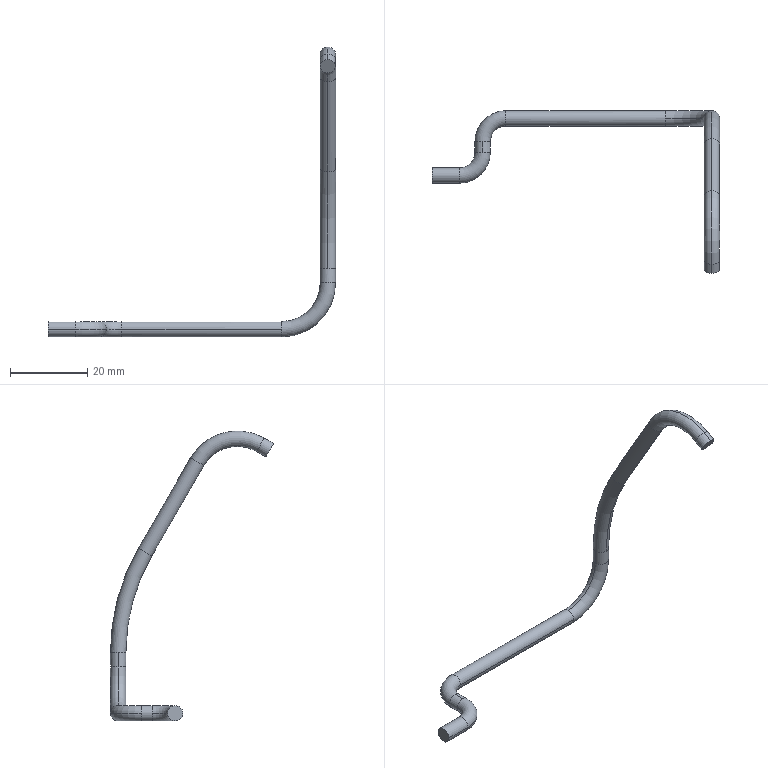Part | SolidWorks | features 3DProfileFeature 2, Sweep 1 | 1 solid | 24 faces | box 74.439 x 42.263 x 75.178 mm | volume 2118 mm3 | cylinder 12 | torus 10 | plane 2 | commonest cylinder face diameters 4 x12
STEP:
#1=CARTESIAN_POINT('',(-50.159,50.824,64.286));
#2=VERTEX_POINT('',#1);
#3=CARTESIAN_POINT('',(-50.154,54.288,66.285));
#4=VERTEX_POINT('',#3);
#5=CARTESIAN_POINT('',(-50.159,52.556,65.286));
#6=DIRECTION('',(0.,-0.4999,0.8661));
#7=DIRECTION('',(1.,0.,0.));
#8=AXIS2_PLACEMENT_3D('',#5,#6,#7);
#9=CIRCLE('',#8,2.);
#10=EDGE_CURVE('',#2,#4,#9,.T.);
#11=ORIENTED_EDGE('',*,*,#10,.T.);
#12=CARTESIAN_POINT('',(-50.191,35.164,71.413));
#13=VERTEX_POINT('',#12);
#14=CARTESIAN_POINT('',(-50.191,42.163,59.287));
#15=DIRECTION('',(1.,-0.00231,-0.001333));
#16=DIRECTION('',(0.00231,1.,0.));
#17=AXIS2_PLACEMENT_3D('',#14,#15,#16);
#18=CIRCLE('',#17,14.);
#19=EDGE_CURVE('',#4,#13,#18,.T.);
#20=ORIENTED_EDGE('',*,*,#19,.T.);
#21=CARTESIAN_POINT('',(-50.191,37.164,67.948));
#22=VERTEX_POINT('',#21);
#23=CARTESIAN_POINT('',(-50.191,36.164,69.681));
#24=DIRECTION('',(-0.002667,-0.8661,-0.4999));
#25=DIRECTION('',(1.,-0.003643,0.0009767));
#26=AXIS2_PLACEMENT_3D('',#23,#24,#25);
#27=CIRCLE('',#26,2.);
#28=EDGE_CURVE('',#22,#13,#27,.T.);
#29=ORIENTED_EDGE('',*,*,#28,.F.);
#30=CARTESIAN_POINT('',(-50.164,50.824,64.286));
#31=VERTEX_POINT('',#30);
#32=CARTESIAN_POINT('',(-50.191,42.163,59.287));
#33=DIRECTION('',(1.,-0.00231,-0.001333));
#34=DIRECTION('',(0.00231,1.,0.));
#35=AXIS2_PLACEMENT_3D('',#32,#33,#34);
#36=CIRCLE('',#35,10.);
#37=EDGE_CURVE('',#31,#22,#36,.T.);
#38=ORIENTED_EDGE('',*,*,#37,.F.);
#39=CARTESIAN_POINT('',(-50.159,52.556,65.286));
#40=DIRECTION('',(0.,-0.4999,0.8661));
#41=DIRECTION('',(1.,0.,0.));
#42=AXIS2_PLACEMENT_3D('',#39,#40,#41);
#43=CIRCLE('',#42,2.);
#44=EDGE_CURVE('',#31,#2,#43,.T.);
#45=ORIENTED_EDGE('',*,*,#44,.T.);
#46=EDGE_LOOP('',(#11,#20,#29,#38,#45));
#47=FACE_OUTER_BOUND('',#46,.T.);
#48=CARTESIAN_POINT('',(-50.191,42.163,59.287));
#49=DIRECTION('',(1.,-0.00231,-0.001333));
#50=DIRECTION('',(0.00231,1.,0.));
#51=AXIS2_PLACEMENT_3D('',#48,#49,#50);
#52=TOROIDAL_SURFACE('',#51,12.,2.);
#53=ADVANCED_FACE('',(#47),#52,.T.);
#54=CARTESIAN_POINT('',(-48.159,73.044,15.858));
#55=VERTEX_POINT('',#54);
#56=CARTESIAN_POINT('',(-50.159,75.044,15.858));
#57=VERTEX_POINT('',#56);
#58=CARTESIAN_POINT('',(-50.159,73.044,15.858));
#59=DIRECTION('',(0.,0.,1.));
#60=DIRECTION('',(1.,0.,0.));
#61=AXIS2_PLACEMENT_3D('',#58,#59,#60);
#62=CIRCLE('',#61,2.);
#63=EDGE_CURVE('',#55,#57,#62,.T.);
#64=ORIENTED_EDGE('',*,*,#63,.T.);
#65=CARTESIAN_POINT('',(-50.159,67.813,42.851));
#66=VERTEX_POINT('',#65);
#67=CARTESIAN_POINT('',(-50.159,21.044,15.858));
#68=DIRECTION('',(1.,0.,0.));
#69=DIRECTION('',(0.,0.,-1.));
#70=AXIS2_PLACEMENT_3D('',#67,#68,#69);
#71=CIRCLE('',#70,54.);
#72=EDGE_CURVE('',#57,#66,#71,.T.);
#73=ORIENTED_EDGE('',*,*,#72,.T.);
#74=CARTESIAN_POINT('',(-50.159,64.349,40.852));
#75=VERTEX_POINT('',#74);
#76=CARTESIAN_POINT('',(-50.159,66.081,41.851));
#77=DIRECTION('',(0.,-0.4999,0.8661));
#78=DIRECTION('',(1.,0.,0.));
#79=AXIS2_PLACEMENT_3D('',#76,#77,#78);
#80=CIRCLE('',#79,2.);
#81=EDGE_CURVE('',#75,#66,#80,.T.);
#82=ORIENTED_EDGE('',*,*,#81,.F.);
#83=CARTESIAN_POINT('',(-50.159,71.044,15.858));
#84=VERTEX_POINT('',#83);
#85=CARTESIAN_POINT('',(-50.159,21.044,15.858));
#86=DIRECTION('',(1.,0.,0.));
#87=DIRECTION('',(0.,0.,-1.));
#88=AXIS2_PLACEMENT_3D('',#85,#86,#87);
#89=CIRCLE('',#88,50.);
#90=EDGE_CURVE('',#84,#75,#89,.T.);
#91=ORIENTED_EDGE('',*,*,#90,.F.);
#92=CARTESIAN_POINT('',(-50.159,73.044,15.858));
#93=DIRECTION('',(0.,0.,1.));
#94=DIRECTION('',(1.,0.,0.));
#95=AXIS2_PLACEMENT_3D('',#92,#93,#94);
#96=CIRCLE('',#95,2.);
#97=EDGE_CURVE('',#84,#55,#96,.T.);
#98=ORIENTED_EDGE('',*,*,#97,.T.);
#99=EDGE_LOOP('',(#64,#73,#82,#91,#98));
#100=FACE_OUTER_BOUND('',#99,.T.);
#101=CARTESIAN_POINT('',(-50.159,21.044,15.858));
#102=DIRECTION('',(1.,0.,0.));
#103=DIRECTION('',(0.,0.,-1.));
#104=AXIS2_PLACEMENT_3D('',#101,#102,#103);
#105=TOROIDAL_SURFACE('',#104,52.,2.);
#106=ADVANCED_FACE('',(#100),#105,.T.);
#107=CARTESIAN_POINT('',(-62.159,71.044,0.1096));
#108=VERTEX_POINT('',#107);
#109=CARTESIAN_POINT('',(-62.159,73.044,-1.89));
#110=VERTEX_POINT('',#109);
#111=CARTESIAN_POINT('',(-62.159,73.044,0.1096));
#112=DIRECTION('',(1.,0.,0.));
#113=DIRECTION('',(0.,0.,-1.));
#114=AXIS2_PLACEMENT_3D('',#111,#112,#113);
#115=CIRCLE('',#114,2.);
#116=EDGE_CURVE('',#108,#110,#115,.T.);
#117=ORIENTED_EDGE('',*,*,#116,.T.);
#118=CARTESIAN_POINT('',(-48.159,73.044,12.11));
#119=VERTEX_POINT('',#118);
#120=CARTESIAN_POINT('',(-62.159,73.044,12.11));
#121=DIRECTION('',(0.,-1.,0.));
#122=DIRECTION('',(0.,0.,-1.));
#123=AXIS2_PLACEMENT_3D('',#120,#121,#122);
#124=CIRCLE('',#123,14.);
#125=EDGE_CURVE('',#110,#119,#124,.T.);
#126=ORIENTED_EDGE('',*,*,#125,.T.);
#127=CARTESIAN_POINT('',(-52.159,73.044,12.11));
#128=VERTEX_POINT('',#127);
#129=CARTESIAN_POINT('',(-50.159,73.044,12.11));
#130=DIRECTION('',(0.,0.,1.));
#131=DIRECTION('',(1.,0.,0.));
#132=AXIS2_PLACEMENT_3D('',#129,#130,#131);
#133=CIRCLE('',#132,2.);
#134=EDGE_CURVE('',#128,#119,#133,.T.);
#135=ORIENTED_EDGE('',*,*,#134,.F.);
#136=CARTESIAN_POINT('',(-62.159,73.044,2.11));
#137=VERTEX_POINT('',#136);
#138=CARTESIAN_POINT('',(-62.159,73.044,12.11));
#139=DIRECTION('',(0.,-1.,0.));
#140=DIRECTION('',(0.,0.,-1.));
#141=AXIS2_PLACEMENT_3D('',#138,#139,#140);
#142=CIRCLE('',#141,10.);
#143=EDGE_CURVE('',#137,#128,#142,.T.);
#144=ORIENTED_EDGE('',*,*,#143,.F.);
#145=CARTESIAN_POINT('',(-62.159,73.044,0.1096));
#146=DIRECTION('',(1.,0.,0.));
#147=DIRECTION('',(0.,0.,-1.));
#148=AXIS2_PLACEMENT_3D('',#145,#146,#147);
#149=CIRCLE('',#148,2.);
#150=EDGE_CURVE('',#137,#108,#149,.T.);
#151=ORIENTED_EDGE('',*,*,#150,.T.);
#152=EDGE_LOOP('',(#117,#126,#135,#144,#151));
#153=FACE_OUTER_BOUND('',#152,.T.);
#154=CARTESIAN_POINT('',(-62.159,73.044,12.11));
#155=DIRECTION('',(0.,-1.,0.));
#156=DIRECTION('',(0.,0.,-1.));
#157=AXIS2_PLACEMENT_3D('',#154,#155,#156);
#158=TOROIDAL_SURFACE('',#157,12.,2.);
#159=ADVANCED_FACE('',(#153),#158,.T.);
#160=CARTESIAN_POINT('',(-109.578,67.044,-1.89));
#161=VERTEX_POINT('',#160);
#162=CARTESIAN_POINT('',(-111.578,67.044,0.1096));
#163=VERTEX_POINT('',#162);
#164=CARTESIAN_POINT('',(-109.578,67.044,0.1096));
#165=DIRECTION('',(0.,1.,0.));
#166=DIRECTION('',(0.,0.,-1.));
#167=AXIS2_PLACEMENT_3D('',#164,#165,#166);
#168=CIRCLE('',#167,2.);
#169=EDGE_CURVE('',#161,#163,#168,.T.);
#170=ORIENTED_EDGE('',*,*,#169,.T.);
#171=CARTESIAN_POINT('',(-103.578,75.044,0.1096));
#172=VERTEX_POINT('',#171);
#173=CARTESIAN_POINT('',(-103.578,67.044,0.1096));
#174=DIRECTION('',(0.,0.,-1.));
#175=DIRECTION('',(-1.,0.,0.));
#176=AXIS2_PLACEMENT_3D('',#173,#174,#175);
#177=CIRCLE('',#176,8.);
#178=EDGE_CURVE('',#163,#172,#177,.T.);
#179=ORIENTED_EDGE('',*,*,#178,.T.);
#180=CARTESIAN_POINT('',(-103.578,71.044,0.1096));
#181=VERTEX_POINT('',#180);
#182=CARTESIAN_POINT('',(-103.578,73.044,0.1096));
#183=DIRECTION('',(1.,0.,0.));
#184=DIRECTION('',(0.,0.,-1.));
#185=AXIS2_PLACEMENT_3D('',#182,#183,#184);
#186=CIRCLE('',#185,2.);
#187=EDGE_CURVE('',#181,#172,#186,.T.);
#188=ORIENTED_EDGE('',*,*,#187,.F.);
#189=CARTESIAN_POINT('',(-107.578,67.044,0.1096));
#190=VERTEX_POINT('',#189);
#191=CARTESIAN_POINT('',(-103.578,67.044,0.1096));
#192=DIRECTION('',(0.,0.,-1.));
#193=DIRECTION('',(-1.,0.,0.));
#194=AXIS2_PLACEMENT_3D('',#191,#192,#193);
#195=CIRCLE('',#194,4.);
#196=EDGE_CURVE('',#190,#181,#195,.T.);
#197=ORIENTED_EDGE('',*,*,#196,.F.);
#198=CARTESIAN_POINT('',(-109.578,67.044,0.1096));
#199=DIRECTION('',(0.,1.,0.));
#200=DIRECTION('',(0.,0.,-1.));
#201=AXIS2_PLACEMENT_3D('',#198,#199,#200);
#202=CIRCLE('',#201,2.);
#203=EDGE_CURVE('',#190,#161,#202,.T.);
#204=ORIENTED_EDGE('',*,*,#203,.T.);
#205=EDGE_LOOP('',(#170,#179,#188,#197,#204));
#206=FACE_OUTER_BOUND('',#205,.T.);
#207=CARTESIAN_POINT('',(-103.578,67.044,0.1096));
#208=DIRECTION('',(0.,0.,-1.));
#209=DIRECTION('',(-1.,0.,0.));
#210=AXIS2_PLACEMENT_3D('',#207,#208,#209);
#211=TOROIDAL_SURFACE('',#210,6.,2.);
#212=ADVANCED_FACE('',(#206),#211,.T.);
#213=CARTESIAN_POINT('',(-115.578,60.264,0.1096));
#214=VERTEX_POINT('',#213);
#215=CARTESIAN_POINT('',(-115.578,56.264,0.1096));
#216=VERTEX_POINT('',#215);
#217=CARTESIAN_POINT('',(-115.578,58.264,0.1096));
#218=DIRECTION('',(1.,0.,0.));
#219=DIRECTION('',(0.,0.,-1.));
#220=AXIS2_PLACEMENT_3D('',#217,#218,#219);
#221=CIRCLE('',#220,2.);
#222=EDGE_CURVE('',#214,#216,#221,.T.);
#223=ORIENTED_EDGE('',*,*,#222,.T.);
#224=CARTESIAN_POINT('',(-107.578,64.264,0.1096));
#225=VERTEX_POINT('',#224);
#226=CARTESIAN_POINT('',(-115.578,64.264,0.1096));
#227=DIRECTION('',(0.,0.,1.));
#228=DIRECTION('',(1.,0.,0.));
#229=AXIS2_PLACEMENT_3D('',#226,#227,#228);
#230=CIRCLE('',#229,8.);
#231=EDGE_CURVE('',#216,#225,#230,.T.);
#232=ORIENTED_EDGE('',*,*,#231,.T.);
#233=CARTESIAN_POINT('',(-109.578,64.264,2.11));
#234=VERTEX_POINT('',#233);
#235=CARTESIAN_POINT('',(-109.578,64.264,0.1096));
#236=DIRECTION('',(0.,1.,0.));
#237=DIRECTION('',(0.,0.,-1.));
#238=AXIS2_PLACEMENT_3D('',#235,#236,#237);
#239=CIRCLE('',#238,2.);
#240=EDGE_CURVE('',#234,#225,#239,.T.);
#241=ORIENTED_EDGE('',*,*,#240,.F.);
#242=CARTESIAN_POINT('',(-111.578,64.264,0.1096));
#243=VERTEX_POINT('',#242);
#244=CARTESIAN_POINT('',(-109.578,64.264,0.1096));
#245=DIRECTION('',(0.,1.,0.));
#246=DIRECTION('',(0.,0.,-1.));
#247=AXIS2_PLACEMENT_3D('',#244,#245,#246);
#248=CIRCLE('',#247,2.);
#249=EDGE_CURVE('',#243,#234,#248,.T.);
#250=ORIENTED_EDGE('',*,*,#249,.F.);
#251=CARTESIAN_POINT('',(-115.578,64.264,0.1096));
#252=DIRECTION('',(0.,0.,1.));
#253=DIRECTION('',(1.,0.,0.));
#254=AXIS2_PLACEMENT_3D('',#251,#252,#253);
#255=CIRCLE('',#254,4.);
#256=EDGE_CURVE('',#214,#243,#255,.T.);
#257=ORIENTED_EDGE('',*,*,#256,.F.);
#258=EDGE_LOOP('',(#223,#232,#241,#250,#257));
#259=FACE_OUTER_BOUND('',#258,.T.);
#260=CARTESIAN_POINT('',(-115.578,64.264,0.1096));
#261=DIRECTION('',(0.,0.,1.));
#262=DIRECTION('',(1.,0.,0.));
#263=AXIS2_PLACEMENT_3D('',#260,#261,#262);
#264=TOROIDAL_SURFACE('',#263,6.,2.);
#265=ADVANCED_FACE('',(#259),#264,.T.);
#266=ORIENTED_EDGE('',*,*,#28,.T.);
#267=CARTESIAN_POINT('',(-50.198,32.78,70.037));
#268=VERTEX_POINT('',#267);
#269=CARTESIAN_POINT('',(-50.191,35.164,71.413));
#270=DIRECTION('',(-0.002667,-0.8661,-0.4999));
#271=VECTOR('',#270,1000.);
#272=LINE('',#269,#271);
#273=EDGE_CURVE('',#13,#268,#272,.T.);
#274=ORIENTED_EDGE('',*,*,#273,.T.);
#275=CARTESIAN_POINT('',(-50.198,34.78,66.572));
#276=VERTEX_POINT('',#275);
#277=CARTESIAN_POINT('',(-50.198,33.78,68.304));
#278=DIRECTION('',(-0.002667,-0.8661,-0.4999));
#279=DIRECTION('',(1.,-0.003643,0.0009767));
#280=AXIS2_PLACEMENT_3D('',#277,#278,#279);
#281=CIRCLE('',#280,2.);
#282=EDGE_CURVE('',#276,#268,#281,.T.);
#283=ORIENTED_EDGE('',*,*,#282,.F.);
#284=CARTESIAN_POINT('',(-50.191,37.164,67.948));
#285=DIRECTION('',(-0.002667,-0.8661,-0.4999));
#286=VECTOR('',#285,1000.);
#287=LINE('',#284,#286);
#288=EDGE_CURVE('',#22,#276,#287,.T.);
#289=ORIENTED_EDGE('',*,*,#288,.F.);
#290=EDGE_LOOP('',(#266,#274,#283,#289));
#291=FACE_OUTER_BOUND('',#290,.T.);
#292=CARTESIAN_POINT('',(-50.191,36.164,69.681));
#293=DIRECTION('',(-0.002667,-0.8661,-0.4999));
#294=DIRECTION('',(0.,0.4999,-0.8661));
#295=AXIS2_PLACEMENT_3D('',#292,#293,#294);
#296=CYLINDRICAL_SURFACE('',#295,2.);
#297=ADVANCED_FACE('',(#291),#296,.T.);
#298=ORIENTED_EDGE('',*,*,#81,.T.);
#299=CARTESIAN_POINT('',(-50.159,54.288,66.285));
#300=VERTEX_POINT('',#299);
#301=CARTESIAN_POINT('',(-50.159,67.813,42.851));
#302=DIRECTION('',(0.,-0.4999,0.8661));
#303=VECTOR('',#302,1000.);
#304=LINE('',#301,#303);
#305=EDGE_CURVE('',#66,#300,#304,.T.);
#306=ORIENTED_EDGE('',*,*,#305,.T.);
#307=CARTESIAN_POINT('',(-50.159,52.556,65.286));
#308=DIRECTION('',(0.,-0.4999,0.8661));
#309=DIRECTION('',(1.,0.,0.));
#310=AXIS2_PLACEMENT_3D('',#307,#308,#309);
#311=CIRCLE('',#310,2.);
#312=EDGE_CURVE('',#4,#300,#311,.T.);
#313=ORIENTED_EDGE('',*,*,#312,.F.);
#314=ORIENTED_EDGE('',*,*,#10,.F.);
#315=CARTESIAN_POINT('',(-50.159,64.349,40.852));
#316=DIRECTION('',(0.,-0.4999,0.8661));
#317=VECTOR('',#316,1000.);
#318=LINE('',#315,#317);
#319=EDGE_CURVE('',#75,#2,#318,.T.);
#320=ORIENTED_EDGE('',*,*,#319,.F.);
#321=EDGE_LOOP('',(#298,#306,#313,#314,#320));
#322=FACE_OUTER_BOUND('',#321,.T.);
#323=CARTESIAN_POINT('',(-50.159,66.081,41.851));
#324=DIRECTION('',(0.,-0.4999,0.8661));
#325=DIRECTION('',(0.,-0.8661,-0.4999));
#326=AXIS2_PLACEMENT_3D('',#323,#324,#325);
#327=CYLINDRICAL_SURFACE('',#326,2.);
#328=ADVANCED_FACE('',(#322),#327,.T.);
#329=CARTESIAN_POINT('',(-50.159,73.044,12.11));
#330=DIRECTION('',(0.,0.,1.));
#331=DIRECTION('',(1.,0.,0.));
#332=AXIS2_PLACEMENT_3D('',#329,#330,#331);
#333=CIRCLE('',#332,2.);
#334=EDGE_CURVE('',#119,#128,#333,.T.);
#335=ORIENTED_EDGE('',*,*,#334,.T.);
#336=CARTESIAN_POINT('',(-52.159,73.044,15.858));
#337=VERTEX_POINT('',#336);
#338=CARTESIAN_POINT('',(-52.159,73.044,12.11));
#339=DIRECTION('',(0.,0.,1.));
#340=VECTOR('',#339,1000.);
#341=LINE('',#338,#340);
#342=EDGE_CURVE('',#128,#337,#341,.T.);
#343=ORIENTED_EDGE('',*,*,#342,.T.);
#344=CARTESIAN_POINT('',(-50.159,73.044,15.858));
#345=DIRECTION('',(0.,0.,1.));
#346=DIRECTION('',(1.,0.,0.));
#347=AXIS2_PLACEMENT_3D('',#344,#345,#346);
#348=CIRCLE('',#347,2.);
#349=EDGE_CURVE('',#57,#337,#348,.T.);
#350=ORIENTED_EDGE('',*,*,#349,.F.);
#351=ORIENTED_EDGE('',*,*,#63,.F.);
#352=CARTESIAN_POINT('',(-48.159,73.044,12.11));
#353=DIRECTION('',(0.,0.,1.));
#354=VECTOR('',#353,1000.);
#355=LINE('',#352,#354);
#356=EDGE_CURVE('',#119,#55,#355,.T.);
#357=ORIENTED_EDGE('',*,*,#356,.F.);
#358=EDGE_LOOP('',(#335,#343,#350,#351,#357));
#359=FACE_OUTER_BOUND('',#358,.T.);
#360=CARTESIAN_POINT('',(-50.159,73.044,12.11));
#361=DIRECTION('',(0.,0.,1.));
#362=DIRECTION('',(1.,0.,0.));
#363=AXIS2_PLACEMENT_3D('',#360,#361,#362);
#364=CYLINDRICAL_SURFACE('',#363,2.);
#365=ADVANCED_FACE('',(#359),#364,.T.);
#366=CARTESIAN_POINT('',(-103.578,73.044,0.1096));
#367=DIRECTION('',(1.,0.,0.));
#368=DIRECTION('',(0.,0.,-1.));
#369=AXIS2_PLACEMENT_3D('',#366,#367,#368);
#370=CIRCLE('',#369,2.);
#371=EDGE_CURVE('',#172,#181,#370,.T.);
#372=ORIENTED_EDGE('',*,*,#371,.T.);
#373=CARTESIAN_POINT('',(-103.578,71.044,0.1096));
#374=DIRECTION('',(1.,0.,0.));
#375=VECTOR('',#374,1000.);
#376=LINE('',#373,#375);
#377=EDGE_CURVE('',#181,#108,#376,.T.);
#378=ORIENTED_EDGE('',*,*,#377,.T.);
#379=ORIENTED_EDGE('',*,*,#150,.F.);
#380=CARTESIAN_POINT('',(-62.159,75.044,0.1096));
#381=VERTEX_POINT('',#380);
#382=CARTESIAN_POINT('',(-62.159,73.044,0.1096));
#383=DIRECTION('',(1.,0.,0.));
#384=DIRECTION('',(0.,0.,-1.));
#385=AXIS2_PLACEMENT_3D('',#382,#383,#384);
#386=CIRCLE('',#385,2.);
#387=EDGE_CURVE('',#381,#137,#386,.T.);
#388=ORIENTED_EDGE('',*,*,#387,.F.);
#389=CARTESIAN_POINT('',(-103.578,75.044,0.1096));
#390=DIRECTION('',(1.,0.,0.));
#391=VECTOR('',#390,1000.);
#392=LINE('',#389,#391);
#393=EDGE_CURVE('',#172,#381,#392,.T.);
#394=ORIENTED_EDGE('',*,*,#393,.F.);
#395=EDGE_LOOP('',(#372,#378,#379,#388,#394));
#396=FACE_OUTER_BOUND('',#395,.T.);
#397=CARTESIAN_POINT('',(-103.578,73.044,0.1096));
#398=DIRECTION('',(1.,0.,0.));
#399=DIRECTION('',(0.,1.,0.));
#400=AXIS2_PLACEMENT_3D('',#397,#398,#399);
#401=CYLINDRICAL_SURFACE('',#400,2.);
#402=ADVANCED_FACE('',(#396),#401,.T.);
#403=ORIENTED_EDGE('',*,*,#240,.T.);
#404=CARTESIAN_POINT('',(-109.578,64.264,-1.89));
#405=VERTEX_POINT('',#404);
#406=CARTESIAN_POINT('',(-109.578,64.264,0.1096));
#407=DIRECTION('',(0.,1.,0.));
#408=DIRECTION('',(0.,0.,-1.));
#409=AXIS2_PLACEMENT_3D('',#406,#407,#408);
#410=CIRCLE('',#409,2.);
#411=EDGE_CURVE('',#225,#405,#410,.T.);
#412=ORIENTED_EDGE('',*,*,#411,.T.);
#413=CARTESIAN_POINT('',(-109.578,64.264,-1.89));
#414=DIRECTION('',(0.,1.,0.));
#415=VECTOR('',#414,1000.);
#416=LINE('',#413,#415);
#417=EDGE_CURVE('',#405,#161,#416,.T.);
#418=ORIENTED_EDGE('',*,*,#417,.T.);
#419=ORIENTED_EDGE('',*,*,#203,.F.);
#420=CARTESIAN_POINT('',(-109.578,67.044,2.11));
#421=VERTEX_POINT('',#420);
#422=CARTESIAN_POINT('',(-109.578,67.044,0.1096));
#423=DIRECTION('',(0.,1.,0.));
#424=DIRECTION('',(0.,0.,-1.));
#425=AXIS2_PLACEMENT_3D('',#422,#423,#424);
#426=CIRCLE('',#425,2.);
#427=EDGE_CURVE('',#421,#190,#426,.T.);
#428=ORIENTED_EDGE('',*,*,#427,.F.);
#429=CARTESIAN_POINT('',(-109.578,64.264,2.11));
#430=DIRECTION('',(0.,1.,0.));
#431=VECTOR('',#430,1000.);
#432=LINE('',#429,#431);
#433=EDGE_CURVE('',#234,#421,#432,.T.);
#434=ORIENTED_EDGE('',*,*,#433,.F.);
#435=EDGE_LOOP('',(#403,#412,#418,#419,#428,#434));
#436=FACE_OUTER_BOUND('',#435,.T.);
#437=CARTESIAN_POINT('',(-109.578,64.264,0.1096));
#438=DIRECTION('',(0.,1.,0.));
#439=DIRECTION('',(0.,0.,1.));
#440=AXIS2_PLACEMENT_3D('',#437,#438,#439);
#441=CYLINDRICAL_SURFACE('',#440,2.);
#442=ADVANCED_FACE('',(#436),#441,.T.);
#443=CARTESIAN_POINT('',(-122.598,60.264,0.1096));
#444=VERTEX_POINT('',#443);
#445=CARTESIAN_POINT('',(-122.598,56.264,0.1096));
#446=VERTEX_POINT('',#445);
#447=CARTESIAN_POINT('',(-122.598,58.264,0.1096));
#448=DIRECTION('',(1.,0.,0.));
#449=DIRECTION('',(0.,0.,-1.));
#450=AXIS2_PLACEMENT_3D('',#447,#448,#449);
#451=CIRCLE('',#450,2.);
#452=EDGE_CURVE('',#444,#446,#451,.T.);
#453=ORIENTED_EDGE('',*,*,#452,.T.);
#454=CARTESIAN_POINT('',(-122.598,56.264,0.1096));
#455=DIRECTION('',(1.,0.,0.));
#456=VECTOR('',#455,1000.);
#457=LINE('',#454,#456);
#458=EDGE_CURVE('',#446,#216,#457,.T.);
#459=ORIENTED_EDGE('',*,*,#458,.T.);
#460=ORIENTED_EDGE('',*,*,#222,.F.);
#461=CARTESIAN_POINT('',(-122.598,60.264,0.1096));
#462=DIRECTION('',(1.,0.,0.));
#463=VECTOR('',#462,1000.);
#464=LINE('',#461,#463);
#465=EDGE_CURVE('',#444,#214,#464,.T.);
#466=ORIENTED_EDGE('',*,*,#465,.F.);
#467=EDGE_LOOP('',(#453,#459,#460,#466));
#468=FACE_OUTER_BOUND('',#467,.T.);
#469=CARTESIAN_POINT('',(-122.598,58.264,0.1096));
#470=DIRECTION('',(1.,0.,0.));
#471=DIRECTION('',(0.,1.,0.));
#472=AXIS2_PLACEMENT_3D('',#469,#470,#471);
#473=CYLINDRICAL_SURFACE('',#472,2.);
#474=ADVANCED_FACE('',(#468),#473,.T.);
#475=ORIENTED_EDGE('',*,*,#273,.F.);
#476=CARTESIAN_POINT('',(-50.191,36.164,69.681));
#477=DIRECTION('',(-0.002667,-0.8661,-0.4999));
#478=DIRECTION('',(1.,-0.003643,0.0009767));
#479=AXIS2_PLACEMENT_3D('',#476,#477,#478);
#480=CIRCLE('',#479,2.);
#481=EDGE_CURVE('',#13,#22,#480,.T.);
#482=ORIENTED_EDGE('',*,*,#481,.T.);
#483=ORIENTED_EDGE('',*,*,#288,.T.);
#484=CARTESIAN_POINT('',(-50.198,33.78,68.304));
#485=DIRECTION('',(-0.002667,-0.8661,-0.4999));
#486=DIRECTION('',(1.,-0.003643,0.0009767));
#487=AXIS2_PLACEMENT_3D('',#484,#485,#486);
#488=CIRCLE('',#487,2.);
#489=EDGE_CURVE('',#268,#276,#488,.T.);
#490=ORIENTED_EDGE('',*,*,#489,.F.);
#491=EDGE_LOOP('',(#475,#482,#483,#490));
#492=FACE_OUTER_BOUND('',#491,.T.);
#493=CARTESIAN_POINT('',(-50.191,36.164,69.681));
#494=DIRECTION('',(-0.002667,-0.8661,-0.4999));
#495=DIRECTION('',(0.,0.4999,-0.8661));
#496=AXIS2_PLACEMENT_3D('',#493,#494,#495);
#497=CYLINDRICAL_SURFACE('',#496,2.);
#498=ADVANCED_FACE('',(#492),#497,.T.);
#499=ORIENTED_EDGE('',*,*,#19,.F.);
#500=ORIENTED_EDGE('',*,*,#312,.T.);
#501=CARTESIAN_POINT('',(-50.159,52.556,65.286));
#502=DIRECTION('',(0.,-0.4999,0.8661));
#503=DIRECTION('',(1.,0.,0.));
#504=AXIS2_PLACEMENT_3D('',#501,#502,#503);
#505=CIRCLE('',#504,2.);
#506=EDGE_CURVE('',#300,#31,#505,.T.);
#507=ORIENTED_EDGE('',*,*,#506,.T.);
#508=ORIENTED_EDGE('',*,*,#37,.T.);
#509=ORIENTED_EDGE('',*,*,#481,.F.);
#510=EDGE_LOOP('',(#499,#500,#507,#508,#509));
#511=FACE_OUTER_BOUND('',#510,.T.);
#512=CARTESIAN_POINT('',(-50.191,42.163,59.287));
#513=DIRECTION('',(1.,-0.00231,-0.001333));
#514=DIRECTION('',(0.00231,1.,0.));
#515=AXIS2_PLACEMENT_3D('',#512,#513,#514);
#516=TOROIDAL_SURFACE('',#515,12.,2.);
#517=ADVANCED_FACE('',(#511),#516,.T.);
#518=ORIENTED_EDGE('',*,*,#305,.F.);
#519=CARTESIAN_POINT('',(-50.159,66.081,41.851));
#520=DIRECTION('',(0.,-0.4999,0.8661));
#521=DIRECTION('',(1.,0.,0.));
#522=AXIS2_PLACEMENT_3D('',#519,#520,#521);
#523=CIRCLE('',#522,2.);
#524=EDGE_CURVE('',#66,#75,#523,.T.);
#525=ORIENTED_EDGE('',*,*,#524,.T.);
#526=ORIENTED_EDGE('',*,*,#319,.T.);
#527=ORIENTED_EDGE('',*,*,#44,.F.);
#528=ORIENTED_EDGE('',*,*,#506,.F.);
#529=EDGE_LOOP('',(#518,#525,#526,#527,#528));
#530=FACE_OUTER_BOUND('',#529,.T.);
#531=CARTESIAN_POINT('',(-50.159,66.081,41.851));
#532=DIRECTION('',(0.,-0.4999,0.8661));
#533=DIRECTION('',(0.,-0.8661,-0.4999));
#534=AXIS2_PLACEMENT_3D('',#531,#532,#533);
#535=CYLINDRICAL_SURFACE('',#534,2.);
#536=ADVANCED_FACE('',(#530),#535,.T.);
#537=ORIENTED_EDGE('',*,*,#72,.F.);
#538=ORIENTED_EDGE('',*,*,#349,.T.);
#539=CARTESIAN_POINT('',(-50.159,73.044,15.858));
#540=DIRECTION('',(0.,0.,1.));
#541=DIRECTION('',(1.,0.,0.));
#542=AXIS2_PLACEMENT_3D('',#539,#540,#541);
#543=CIRCLE('',#542,2.);
#544=EDGE_CURVE('',#337,#84,#543,.T.);
#545=ORIENTED_EDGE('',*,*,#544,.T.);
#546=ORIENTED_EDGE('',*,*,#90,.T.);
#547=ORIENTED_EDGE('',*,*,#524,.F.);
#548=EDGE_LOOP('',(#537,#538,#545,#546,#547));
#549=FACE_OUTER_BOUND('',#548,.T.);
#550=CARTESIAN_POINT('',(-50.159,21.044,15.858));
#551=DIRECTION('',(1.,0.,0.));
#552=DIRECTION('',(0.,0.,-1.));
#553=AXIS2_PLACEMENT_3D('',#550,#551,#552);
#554=TOROIDAL_SURFACE('',#553,52.,2.);
#555=ADVANCED_FACE('',(#549),#554,.T.);
#556=ORIENTED_EDGE('',*,*,#342,.F.);
#557=ORIENTED_EDGE('',*,*,#134,.T.);
#558=ORIENTED_EDGE('',*,*,#356,.T.);
#559=ORIENTED_EDGE('',*,*,#97,.F.);
#560=ORIENTED_EDGE('',*,*,#544,.F.);
#561=EDGE_LOOP('',(#556,#557,#558,#559,#560));
#562=FACE_OUTER_BOUND('',#561,.T.);
#563=CARTESIAN_POINT('',(-50.159,73.044,12.11));
#564=DIRECTION('',(0.,0.,1.));
#565=DIRECTION('',(1.,0.,0.));
#566=AXIS2_PLACEMENT_3D('',#563,#564,#565);
#567=CYLINDRICAL_SURFACE('',#566,2.);
#568=ADVANCED_FACE('',(#562),#567,.T.);
#569=ORIENTED_EDGE('',*,*,#125,.F.);
#570=CARTESIAN_POINT('',(-62.159,73.044,0.1096));
#571=DIRECTION('',(1.,0.,0.));
#572=DIRECTION('',(0.,0.,-1.));
#573=AXIS2_PLACEMENT_3D('',#570,#571,#572);
#574=CIRCLE('',#573,2.);
#575=EDGE_CURVE('',#110,#381,#574,.T.);
#576=ORIENTED_EDGE('',*,*,#575,.T.);
#577=ORIENTED_EDGE('',*,*,#387,.T.);
#578=ORIENTED_EDGE('',*,*,#143,.T.);
#579=ORIENTED_EDGE('',*,*,#334,.F.);
#580=EDGE_LOOP('',(#569,#576,#577,#578,#579));
#581=FACE_OUTER_BOUND('',#580,.T.);
#582=CARTESIAN_POINT('',(-62.159,73.044,12.11));
#583=DIRECTION('',(0.,-1.,0.));
#584=DIRECTION('',(0.,0.,-1.));
#585=AXIS2_PLACEMENT_3D('',#582,#583,#584);
#586=TOROIDAL_SURFACE('',#585,12.,2.);
#587=ADVANCED_FACE('',(#581),#586,.T.);
#588=ORIENTED_EDGE('',*,*,#377,.F.);
#589=ORIENTED_EDGE('',*,*,#187,.T.);
#590=ORIENTED_EDGE('',*,*,#393,.T.);
#591=ORIENTED_EDGE('',*,*,#575,.F.);
#592=ORIENTED_EDGE('',*,*,#116,.F.);
#593=EDGE_LOOP('',(#588,#589,#590,#591,#592));
#594=FACE_OUTER_BOUND('',#593,.T.);
#595=CARTESIAN_POINT('',(-103.578,73.044,0.1096));
#596=DIRECTION('',(1.,0.,0.));
#597=DIRECTION('',(0.,1.,0.));
#598=AXIS2_PLACEMENT_3D('',#595,#596,#597);
#599=CYLINDRICAL_SURFACE('',#598,2.);
#600=ADVANCED_FACE('',(#594),#599,.T.);
#601=ORIENTED_EDGE('',*,*,#178,.F.);
#602=CARTESIAN_POINT('',(-109.578,67.044,0.1096));
#603=DIRECTION('',(0.,1.,0.));
#604=DIRECTION('',(0.,0.,-1.));
#605=AXIS2_PLACEMENT_3D('',#602,#603,#604);
#606=CIRCLE('',#605,2.);
#607=EDGE_CURVE('',#163,#421,#606,.T.);
#608=ORIENTED_EDGE('',*,*,#607,.T.);
#609=ORIENTED_EDGE('',*,*,#427,.T.);
#610=ORIENTED_EDGE('',*,*,#196,.T.);
#611=ORIENTED_EDGE('',*,*,#371,.F.);
#612=EDGE_LOOP('',(#601,#608,#609,#610,#611));
#613=FACE_OUTER_BOUND('',#612,.T.);
#614=CARTESIAN_POINT('',(-103.578,67.044,0.1096));
#615=DIRECTION('',(0.,0.,-1.));
#616=DIRECTION('',(-1.,0.,0.));
#617=AXIS2_PLACEMENT_3D('',#614,#615,#616);
#618=TOROIDAL_SURFACE('',#617,6.,2.);
#619=ADVANCED_FACE('',(#613),#618,.T.);
#620=ORIENTED_EDGE('',*,*,#417,.F.);
#621=CARTESIAN_POINT('',(-109.578,64.264,0.1096));
#622=DIRECTION('',(0.,1.,0.));
#623=DIRECTION('',(0.,0.,-1.));
#624=AXIS2_PLACEMENT_3D('',#621,#622,#623);
#625=CIRCLE('',#624,2.);
#626=EDGE_CURVE('',#405,#243,#625,.T.);
#627=ORIENTED_EDGE('',*,*,#626,.T.);
#628=ORIENTED_EDGE('',*,*,#249,.T.);
#629=ORIENTED_EDGE('',*,*,#433,.T.);
#630=ORIENTED_EDGE('',*,*,#607,.F.);
#631=ORIENTED_EDGE('',*,*,#169,.F.);
#632=EDGE_LOOP('',(#620,#627,#628,#629,#630,#631));
#633=FACE_OUTER_BOUND('',#632,.T.);
#634=CARTESIAN_POINT('',(-109.578,64.264,0.1096));
#635=DIRECTION('',(0.,1.,0.));
#636=DIRECTION('',(0.,0.,1.));
#637=AXIS2_PLACEMENT_3D('',#634,#635,#636);
#638=CYLINDRICAL_SURFACE('',#637,2.);
#639=ADVANCED_FACE('',(#633),#638,.T.);
#640=ORIENTED_EDGE('',*,*,#231,.F.);
#641=CARTESIAN_POINT('',(-115.578,58.264,0.1096));
#642=DIRECTION('',(1.,0.,0.));
#643=DIRECTION('',(0.,0.,-1.));
#644=AXIS2_PLACEMENT_3D('',#641,#642,#643);
#645=CIRCLE('',#644,2.);
#646=EDGE_CURVE('',#216,#214,#645,.T.);
#647=ORIENTED_EDGE('',*,*,#646,.T.);
#648=ORIENTED_EDGE('',*,*,#256,.T.);
#649=ORIENTED_EDGE('',*,*,#626,.F.);
#650=ORIENTED_EDGE('',*,*,#411,.F.);
#651=EDGE_LOOP('',(#640,#647,#648,#649,#650));
#652=FACE_OUTER_BOUND('',#651,.T.);
#653=CARTESIAN_POINT('',(-115.578,64.264,0.1096));
#654=DIRECTION('',(0.,0.,1.));
#655=DIRECTION('',(1.,0.,0.));
#656=AXIS2_PLACEMENT_3D('',#653,#654,#655);
#657=TOROIDAL_SURFACE('',#656,6.,2.);
#658=ADVANCED_FACE('',(#652),#657,.T.);
#659=ORIENTED_EDGE('',*,*,#458,.F.);
#660=CARTESIAN_POINT('',(-122.598,58.264,0.1096));
#661=DIRECTION('',(1.,0.,0.));
#662=DIRECTION('',(0.,0.,-1.));
#663=AXIS2_PLACEMENT_3D('',#660,#661,#662);
#664=CIRCLE('',#663,2.);
#665=EDGE_CURVE('',#446,#444,#664,.T.);
#666=ORIENTED_EDGE('',*,*,#665,.T.);
#667=ORIENTED_EDGE('',*,*,#465,.T.);
#668=ORIENTED_EDGE('',*,*,#646,.F.);
#669=EDGE_LOOP('',(#659,#666,#667,#668));
#670=FACE_OUTER_BOUND('',#669,.T.);
#671=CARTESIAN_POINT('',(-122.598,58.264,0.1096));
#672=DIRECTION('',(1.,0.,0.));
#673=DIRECTION('',(0.,1.,0.));
#674=AXIS2_PLACEMENT_3D('',#671,#672,#673);
#675=CYLINDRICAL_SURFACE('',#674,2.);
#676=ADVANCED_FACE('',(#670),#675,.T.);
#677=ORIENTED_EDGE('',*,*,#282,.T.);
#678=ORIENTED_EDGE('',*,*,#489,.T.);
#679=EDGE_LOOP('',(#677,#678));
#680=FACE_OUTER_BOUND('',#679,.T.);
#681=CARTESIAN_POINT('',(-50.198,33.78,68.304));
#682=DIRECTION('',(-0.002667,-0.8661,-0.4999));
#683=DIRECTION('',(1.,-0.003643,0.0009767));
#684=AXIS2_PLACEMENT_3D('',#681,#682,#683);
#685=PLANE('',#684);
#686=ADVANCED_FACE('',(#680),#685,.T.);
#687=ORIENTED_EDGE('',*,*,#452,.F.);
#688=ORIENTED_EDGE('',*,*,#665,.F.);
#689=EDGE_LOOP('',(#687,#688));
#690=FACE_OUTER_BOUND('',#689,.T.);
#691=CARTESIAN_POINT('',(-122.598,58.264,0.1096));
#692=DIRECTION('',(1.,0.,0.));
#693=DIRECTION('',(0.,0.,-1.));
#694=AXIS2_PLACEMENT_3D('',#691,#692,#693);
#695=PLANE('',#694);
#696=ADVANCED_FACE('',(#690),#695,.F.);
#697=CLOSED_SHELL('',(#53,#106,#159,#212,#265,#297,#328,#365,#402,#442,#474,#498,#517,#536,#555,#568,#587,#600,#619,#639,#658,#676,#686,#696));
#698=MANIFOLD_SOLID_BREP('',#697);
#699=CARTESIAN_POINT('',(0.,0.,0.));
#700=DIRECTION('',(0.,0.,1.));
#701=DIRECTION('',(1.,0.,0.));
#702=AXIS2_PLACEMENT_3D('',#699,#700,#701);
#703=(LENGTH_UNIT()NAMED_UNIT(*)SI_UNIT(.MILLI.,.METRE.));
#704=UNCERTAINTY_MEASURE_WITH_UNIT(LENGTH_MEASURE(0.00001),#703,'','');
#705=(NAMED_UNIT(*)PLANE_ANGLE_UNIT()SI_UNIT($,.RADIAN.));
#706=(NAMED_UNIT(*)SI_UNIT($,.STERADIAN.)SOLID_ANGLE_UNIT());
#707=(GEOMETRIC_REPRESENTATION_CONTEXT(3)GLOBAL_UNCERTAINTY_ASSIGNED_CONTEXT((#704))GLOBAL_UNIT_ASSIGNED_CONTEXT((#703,#705,#706))REPRESENTATION_CONTEXT('',''));
#708=ADVANCED_BREP_SHAPE_REPRESENTATION('',(#698,#702),#707);